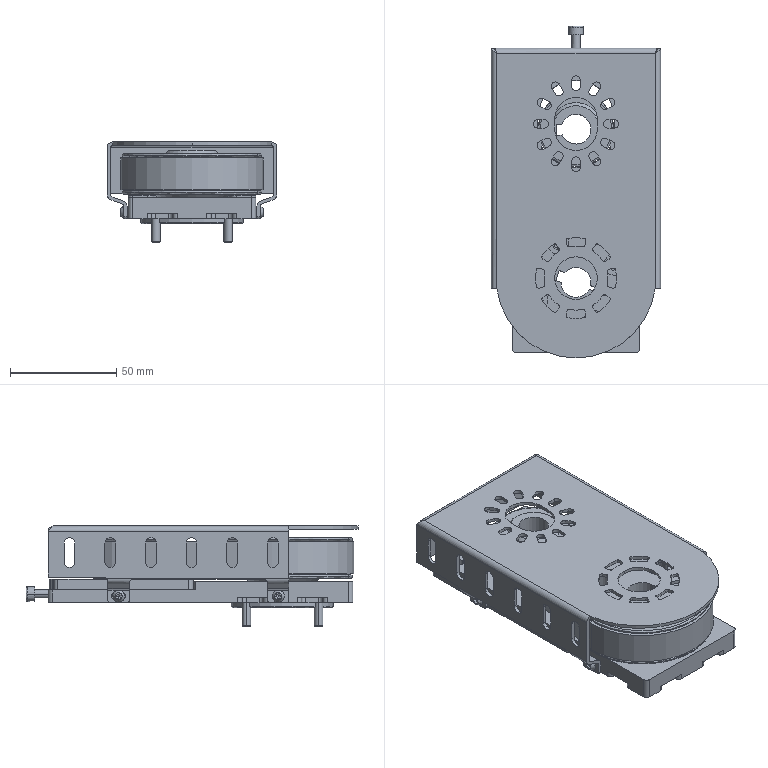Part | SolidWorks | features BaseBody 3, MoveFace 2, ICE 1 | 3 solids | 1501 faces | box 79.5 x 156 x 47 mm | volume 158160 mm3 | cylinder 848 | plane 570 | cone 49 | spline 34 | commonest cylinder face diameters 0.8 x246 2.98 x135 4 x96 63.7 x67 2 x59 5 x53